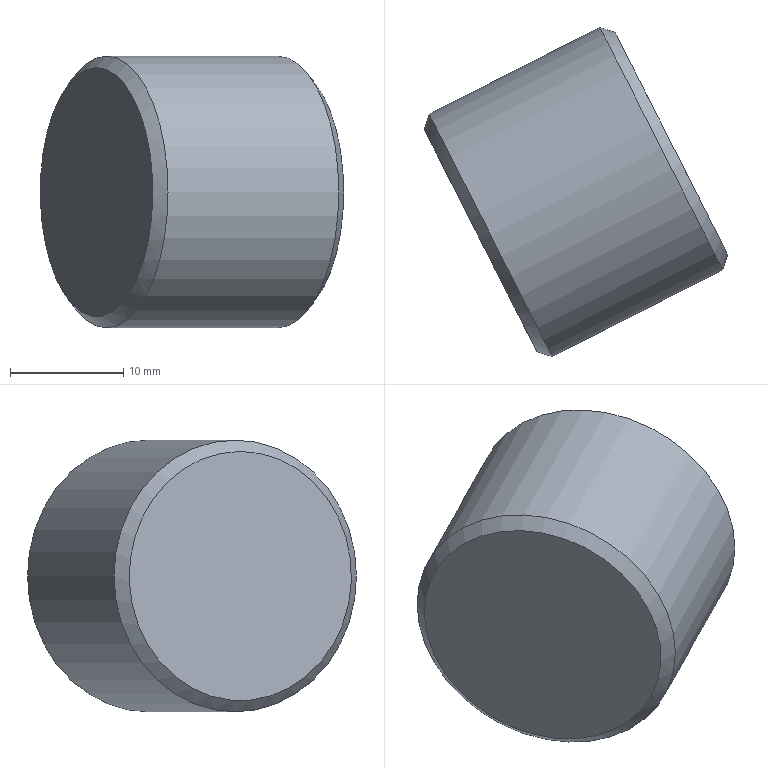Part | STEP file | solid 197 | 1 solid | 12 faces | box 26.803 x 29.047 x 24 mm | volume 6695 mm3 | plane 9 | cone 2 | cylinder 1 | commonest cylinder face diameters 24 x1